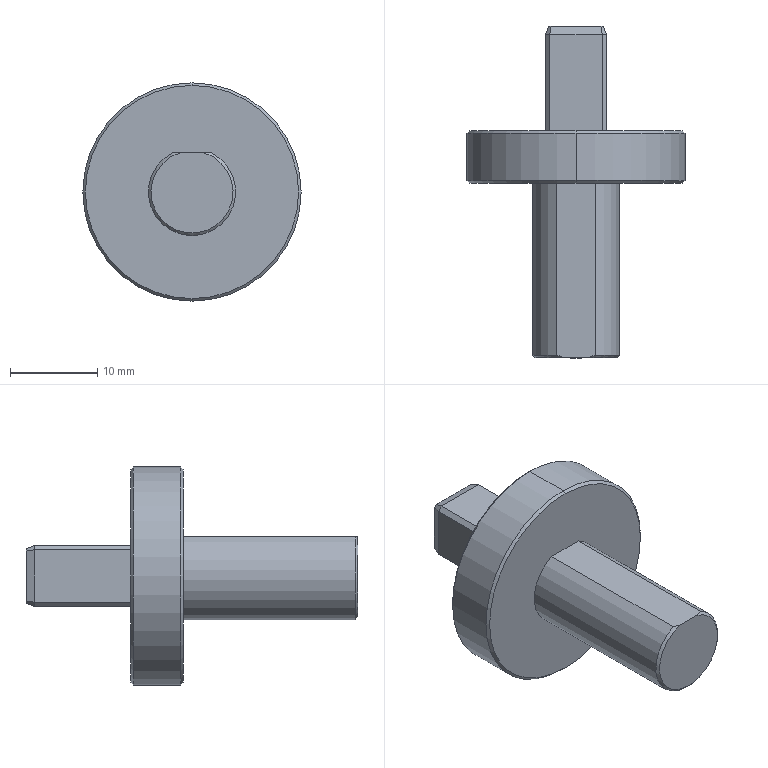Part | NX | features BREP 1 | 1 solid | 29 faces | box 25 x 38 x 25 mm | volume 5056 mm3 | plane 21 | cone 5 | cylinder 3 | commonest cylinder face diameters 25 x2 10 x1
STEP:
#1=CARTESIAN_POINT('',(0.,20.,-12.2));
#2=VERTEX_POINT('',#1);
#3=CARTESIAN_POINT('',(0.,20.,12.2));
#4=VERTEX_POINT('',#3);
#5=CARTESIAN_POINT('',(0.,20.,0.));
#6=DIRECTION('',(0.,-1.,0.));
#7=DIRECTION('',(0.,0.,1.));
#8=AXIS2_PLACEMENT_3D('',#5,#6,#7);
#9=CIRCLE('',#8,12.2);
#10=EDGE_CURVE('',#2,#4,#9,.T.);
#11=ORIENTED_EDGE('',*,*,#10,.F.);
#12=CARTESIAN_POINT('',(0.,20.3,-12.5));
#13=VERTEX_POINT('',#12);
#14=CARTESIAN_POINT('',(0.,20.3,-12.5));
#15=DIRECTION('',(0.,0.7071,-0.7071));
#16=VECTOR('',#15,1000.);
#17=LINE('',#14,#16);
#18=EDGE_CURVE('',#2,#13,#17,.T.);
#19=ORIENTED_EDGE('',*,*,#18,.T.);
#20=CARTESIAN_POINT('',(0.,20.3,12.5));
#21=VERTEX_POINT('',#20);
#22=CARTESIAN_POINT('',(0.,20.3,0.));
#23=DIRECTION('',(0.,1.,0.));
#24=DIRECTION('',(0.,0.,1.));
#25=AXIS2_PLACEMENT_3D('',#22,#23,#24);
#26=CIRCLE('',#25,12.5);
#27=EDGE_CURVE('',#21,#13,#26,.T.);
#28=ORIENTED_EDGE('',*,*,#27,.F.);
#29=CARTESIAN_POINT('',(0.,20.3,12.5));
#30=DIRECTION('',(0.,0.7071,0.7071));
#31=VECTOR('',#30,1000.);
#32=LINE('',#29,#31);
#33=EDGE_CURVE('',#4,#21,#32,.T.);
#34=ORIENTED_EDGE('',*,*,#33,.F.);
#35=EDGE_LOOP('',(#11,#19,#28,#34));
#36=FACE_BOUND('',#35,.T.);
#37=CARTESIAN_POINT('',(0.,20.3,0.));
#38=DIRECTION('',(0.,1.,0.));
#39=DIRECTION('',(0.,0.,-1.));
#40=AXIS2_PLACEMENT_3D('',#37,#38,#39);
#41=CONICAL_SURFACE('',#40,12.5,0.7854);
#42=ADVANCED_FACE('',(#36),#41,.T.);
#43=CARTESIAN_POINT('',(0.,26.,12.2));
#44=VERTEX_POINT('',#43);
#45=CARTESIAN_POINT('',(0.,26.,-12.2));
#46=VERTEX_POINT('',#45);
#47=CARTESIAN_POINT('',(0.,26.,0.));
#48=DIRECTION('',(0.,1.,0.));
#49=DIRECTION('',(0.,0.,1.));
#50=AXIS2_PLACEMENT_3D('',#47,#48,#49);
#51=CIRCLE('',#50,12.2);
#52=EDGE_CURVE('',#44,#46,#51,.T.);
#53=ORIENTED_EDGE('',*,*,#52,.F.);
#54=CARTESIAN_POINT('',(0.,25.7,12.5));
#55=VERTEX_POINT('',#54);
#56=CARTESIAN_POINT('',(0.,26.,12.2));
#57=DIRECTION('',(0.,-0.7071,0.7071));
#58=VECTOR('',#57,1000.);
#59=LINE('',#56,#58);
#60=EDGE_CURVE('',#55,#44,#59,.F.);
#61=ORIENTED_EDGE('',*,*,#60,.F.);
#62=CARTESIAN_POINT('',(0.,25.7,-12.5));
#63=VERTEX_POINT('',#62);
#64=CARTESIAN_POINT('',(0.,25.7,0.));
#65=DIRECTION('',(0.,-1.,0.));
#66=DIRECTION('',(0.,0.,1.));
#67=AXIS2_PLACEMENT_3D('',#64,#65,#66);
#68=CIRCLE('',#67,12.5);
#69=EDGE_CURVE('',#63,#55,#68,.T.);
#70=ORIENTED_EDGE('',*,*,#69,.F.);
#71=CARTESIAN_POINT('',(0.,26.,-12.2));
#72=DIRECTION('',(0.,-0.7071,-0.7071));
#73=VECTOR('',#72,1000.);
#74=LINE('',#71,#73);
#75=EDGE_CURVE('',#63,#46,#74,.F.);
#76=ORIENTED_EDGE('',*,*,#75,.T.);
#77=EDGE_LOOP('',(#53,#61,#70,#76));
#78=FACE_BOUND('',#77,.T.);
#79=CARTESIAN_POINT('',(0.,26.,0.));
#80=DIRECTION('',(0.,-1.,0.));
#81=DIRECTION('',(0.,0.,1.));
#82=AXIS2_PLACEMENT_3D('',#79,#80,#81);
#83=CONICAL_SURFACE('',#82,12.2,0.7854);
#84=ADVANCED_FACE('',(#78),#83,.T.);
#85=ORIENTED_EDGE('',*,*,#27,.T.);
#86=CARTESIAN_POINT('',(0.,66.923,-12.5));
#87=DIRECTION('',(0.,1.,0.));
#88=VECTOR('',#87,1000.);
#89=LINE('',#86,#88);
#90=EDGE_CURVE('',#13,#63,#89,.T.);
#91=ORIENTED_EDGE('',*,*,#90,.T.);
#92=ORIENTED_EDGE('',*,*,#69,.T.);
#93=CARTESIAN_POINT('',(0.,66.923,12.5));
#94=DIRECTION('',(0.,1.,0.));
#95=VECTOR('',#94,1000.);
#96=LINE('',#93,#95);
#97=EDGE_CURVE('',#21,#55,#96,.T.);
#98=ORIENTED_EDGE('',*,*,#97,.F.);
#99=EDGE_LOOP('',(#85,#91,#92,#98));
#100=FACE_BOUND('',#99,.T.);
#101=CARTESIAN_POINT('',(0.,66.923,0.));
#102=DIRECTION('',(0.,1.,0.));
#103=DIRECTION('',(0.,0.,-1.));
#104=AXIS2_PLACEMENT_3D('',#101,#102,#103);
#105=CYLINDRICAL_SURFACE('',#104,12.5);
#106=ADVANCED_FACE('',(#100),#105,.T.);
#107=ORIENTED_EDGE('',*,*,#90,.F.);
#108=CARTESIAN_POINT('',(0.,20.3,0.));
#109=DIRECTION('',(0.,1.,0.));
#110=DIRECTION('',(0.,0.,1.));
#111=AXIS2_PLACEMENT_3D('',#108,#109,#110);
#112=CIRCLE('',#111,12.5);
#113=EDGE_CURVE('',#13,#21,#112,.T.);
#114=ORIENTED_EDGE('',*,*,#113,.T.);
#115=ORIENTED_EDGE('',*,*,#97,.T.);
#116=CARTESIAN_POINT('',(0.,25.7,0.));
#117=DIRECTION('',(0.,-1.,0.));
#118=DIRECTION('',(0.,0.,1.));
#119=AXIS2_PLACEMENT_3D('',#116,#117,#118);
#120=CIRCLE('',#119,12.5);
#121=EDGE_CURVE('',#55,#63,#120,.T.);
#122=ORIENTED_EDGE('',*,*,#121,.T.);
#123=EDGE_LOOP('',(#107,#114,#115,#122));
#124=FACE_BOUND('',#123,.T.);
#125=CARTESIAN_POINT('',(0.,66.923,0.));
#126=DIRECTION('',(0.,1.,0.));
#127=DIRECTION('',(0.,0.,-1.));
#128=AXIS2_PLACEMENT_3D('',#125,#126,#127);
#129=CYLINDRICAL_SURFACE('',#128,12.5);
#130=ADVANCED_FACE('',(#124),#129,.T.);
#131=CARTESIAN_POINT('',(0.,20.,0.));
#132=DIRECTION('',(0.,-1.,0.));
#133=DIRECTION('',(0.,0.,1.));
#134=AXIS2_PLACEMENT_3D('',#131,#132,#133);
#135=CIRCLE('',#134,12.2);
#136=EDGE_CURVE('',#4,#2,#135,.T.);
#137=ORIENTED_EDGE('',*,*,#136,.T.);
#138=ORIENTED_EDGE('',*,*,#10,.T.);
#139=EDGE_LOOP('',(#137,#138));
#140=FACE_BOUND('',#139,.T.);
#141=CARTESIAN_POINT('',(2.179,20.,4.5));
#142=VERTEX_POINT('',#141);
#143=CARTESIAN_POINT('',(-2.179,20.,4.5));
#144=VERTEX_POINT('',#143);
#145=CARTESIAN_POINT('',(0.,20.,0.));
#146=DIRECTION('',(0.,1.,0.));
#147=DIRECTION('',(0.,0.,1.));
#148=AXIS2_PLACEMENT_3D('',#145,#146,#147);
#149=CIRCLE('',#148,5.);
#150=EDGE_CURVE('',#142,#144,#149,.T.);
#151=ORIENTED_EDGE('',*,*,#150,.T.);
#152=CARTESIAN_POINT('',(-2.179,20.,4.5));
#153=DIRECTION('',(1.,0.,0.));
#154=VECTOR('',#153,1000.);
#155=LINE('',#152,#154);
#156=EDGE_CURVE('',#144,#142,#155,.T.);
#157=ORIENTED_EDGE('',*,*,#156,.T.);
#158=EDGE_LOOP('',(#151,#157));
#159=FACE_BOUND('',#158,.T.);
#160=CARTESIAN_POINT('',(12.5,20.,0.));
#161=DIRECTION('',(0.,1.,0.));
#162=DIRECTION('',(0.,0.,-1.));
#163=AXIS2_PLACEMENT_3D('',#160,#161,#162);
#164=PLANE('',#163);
#165=ADVANCED_FACE('',(#140,#159),#164,.F.);
#166=CARTESIAN_POINT('',(2.179,0.3,4.5));
#167=VERTEX_POINT('',#166);
#168=CARTESIAN_POINT('',(2.179,24.387,4.5));
#169=DIRECTION('',(0.,-1.,0.));
#170=VECTOR('',#169,1000.);
#171=LINE('',#168,#170);
#172=EDGE_CURVE('',#167,#142,#171,.F.);
#173=ORIENTED_EDGE('',*,*,#172,.F.);
#174=CARTESIAN_POINT('',(-2.179,0.3,4.5));
#175=VERTEX_POINT('',#174);
#176=CARTESIAN_POINT('',(0.,0.3,0.));
#177=DIRECTION('',(0.,1.,0.));
#178=DIRECTION('',(0.,0.,1.));
#179=AXIS2_PLACEMENT_3D('',#176,#177,#178);
#180=CIRCLE('',#179,5.);
#181=EDGE_CURVE('',#167,#175,#180,.T.);
#182=ORIENTED_EDGE('',*,*,#181,.T.);
#183=CARTESIAN_POINT('',(-2.179,24.387,4.5));
#184=DIRECTION('',(0.,-1.,0.));
#185=VECTOR('',#184,1000.);
#186=LINE('',#183,#185);
#187=EDGE_CURVE('',#175,#144,#186,.F.);
#188=ORIENTED_EDGE('',*,*,#187,.T.);
#189=ORIENTED_EDGE('',*,*,#150,.F.);
#190=EDGE_LOOP('',(#173,#182,#188,#189));
#191=FACE_BOUND('',#190,.T.);
#192=CARTESIAN_POINT('',(0.,66.923,0.));
#193=DIRECTION('',(0.,1.,0.));
#194=DIRECTION('',(0.,0.,-1.));
#195=AXIS2_PLACEMENT_3D('',#192,#193,#194);
#196=CYLINDRICAL_SURFACE('',#195,5.);
#197=ADVANCED_FACE('',(#191),#196,.T.);
#198=CARTESIAN_POINT('',(-1.356,0.,4.5));
#199=VERTEX_POINT('',#198);
#200=CARTESIAN_POINT('',(1.356,0.,4.5));
#201=VERTEX_POINT('',#200);
#202=CARTESIAN_POINT('',(-2.179,0.,4.5));
#203=DIRECTION('',(1.,0.,0.));
#204=VECTOR('',#203,1000.);
#205=LINE('',#202,#204);
#206=EDGE_CURVE('',#199,#201,#205,.T.);
#207=ORIENTED_EDGE('',*,*,#206,.F.);
#208=CARTESIAN_POINT('',(0.,0.,0.));
#209=DIRECTION('',(0.,-1.,0.));
#210=DIRECTION('',(0.,0.,1.));
#211=AXIS2_PLACEMENT_3D('',#208,#209,#210);
#212=CIRCLE('',#211,4.7);
#213=EDGE_CURVE('',#199,#201,#212,.T.);
#214=ORIENTED_EDGE('',*,*,#213,.T.);
#215=EDGE_LOOP('',(#207,#214));
#216=FACE_BOUND('',#215,.T.);
#217=CARTESIAN_POINT('',(5.,0.,0.));
#218=DIRECTION('',(0.,1.,0.));
#219=DIRECTION('',(0.,0.,-1.));
#220=AXIS2_PLACEMENT_3D('',#217,#218,#219);
#221=PLANE('',#220);
#222=ADVANCED_FACE('',(#216),#221,.F.);
#223=ORIENTED_EDGE('',*,*,#187,.F.);
#224=CARTESIAN_POINT('',(-2.179,0.3,4.5));
#225=CARTESIAN_POINT('',(-1.911,0.1831,4.5));
#226=CARTESIAN_POINT('',(-1.638,0.08116,4.5));
#227=CARTESIAN_POINT('',(-1.356,0.,4.5));
#228=B_SPLINE_CURVE_WITH_KNOTS('',3,(#224,#225,#226,#227),.UNSPECIFIED.,.F.,.F.,(4,4),(0.,0.000876),.UNSPECIFIED.);
#229=EDGE_CURVE('',#175,#199,#228,.T.);
#230=ORIENTED_EDGE('',*,*,#229,.T.);
#231=ORIENTED_EDGE('',*,*,#206,.T.);
#232=CARTESIAN_POINT('',(1.356,0.,4.5));
#233=CARTESIAN_POINT('',(1.638,0.08116,4.5));
#234=CARTESIAN_POINT('',(1.911,0.1831,4.5));
#235=CARTESIAN_POINT('',(2.179,0.3,4.5));
#236=B_SPLINE_CURVE_WITH_KNOTS('',3,(#232,#233,#234,#235),.UNSPECIFIED.,.F.,.F.,(4,4),(0.,0.000876),.UNSPECIFIED.);
#237=EDGE_CURVE('',#201,#167,#236,.T.);
#238=ORIENTED_EDGE('',*,*,#237,.T.);
#239=ORIENTED_EDGE('',*,*,#172,.T.);
#240=ORIENTED_EDGE('',*,*,#156,.F.);
#241=EDGE_LOOP('',(#223,#230,#231,#238,#239,#240));
#242=FACE_BOUND('',#241,.T.);
#243=CARTESIAN_POINT('',(-2.179,24.387,4.5));
#244=DIRECTION('',(0.,0.,-1.));
#245=DIRECTION('',(1.,0.,0.));
#246=AXIS2_PLACEMENT_3D('',#243,#244,#245);
#247=PLANE('',#246);
#248=ADVANCED_FACE('',(#242),#247,.F.);
#249=CARTESIAN_POINT('',(0.,26.,0.));
#250=DIRECTION('',(0.,1.,0.));
#251=DIRECTION('',(0.,0.,1.));
#252=AXIS2_PLACEMENT_3D('',#249,#250,#251);
#253=CIRCLE('',#252,12.2);
#254=EDGE_CURVE('',#46,#44,#253,.T.);
#255=ORIENTED_EDGE('',*,*,#254,.T.);
#256=ORIENTED_EDGE('',*,*,#52,.T.);
#257=EDGE_LOOP('',(#255,#256));
#258=FACE_BOUND('',#257,.T.);
#259=CARTESIAN_POINT('',(-3.,26.,3.5));
#260=VERTEX_POINT('',#259);
#261=CARTESIAN_POINT('',(3.,26.,3.5));
#262=VERTEX_POINT('',#261);
#263=CARTESIAN_POINT('',(-3.5,26.,3.5));
#264=DIRECTION('',(1.,0.,0.));
#265=VECTOR('',#264,1000.);
#266=LINE('',#263,#265);
#267=EDGE_CURVE('',#260,#262,#266,.T.);
#268=ORIENTED_EDGE('',*,*,#267,.F.);
#269=CARTESIAN_POINT('',(-3.5,26.,3.));
#270=VERTEX_POINT('',#269);
#271=CARTESIAN_POINT('',(-3.5,26.,3.));
#272=DIRECTION('',(-0.7071,0.,-0.7071));
#273=VECTOR('',#272,1000.);
#274=LINE('',#271,#273);
#275=EDGE_CURVE('',#260,#270,#274,.T.);
#276=ORIENTED_EDGE('',*,*,#275,.T.);
#277=CARTESIAN_POINT('',(-3.5,26.,-3.));
#278=VERTEX_POINT('',#277);
#279=CARTESIAN_POINT('',(-3.5,26.,-3.5));
#280=DIRECTION('',(0.,0.,1.));
#281=VECTOR('',#280,1000.);
#282=LINE('',#279,#281);
#283=EDGE_CURVE('',#278,#270,#282,.T.);
#284=ORIENTED_EDGE('',*,*,#283,.F.);
#285=CARTESIAN_POINT('',(-3.,26.,-3.5));
#286=VERTEX_POINT('',#285);
#287=CARTESIAN_POINT('',(-3.,26.,-3.5));
#288=DIRECTION('',(0.7071,0.,-0.7071));
#289=VECTOR('',#288,1000.);
#290=LINE('',#287,#289);
#291=EDGE_CURVE('',#278,#286,#290,.T.);
#292=ORIENTED_EDGE('',*,*,#291,.T.);
#293=CARTESIAN_POINT('',(3.,26.,-3.5));
#294=VERTEX_POINT('',#293);
#295=CARTESIAN_POINT('',(-3.5,26.,-3.5));
#296=DIRECTION('',(-1.,0.,0.));
#297=VECTOR('',#296,1000.);
#298=LINE('',#295,#297);
#299=EDGE_CURVE('',#294,#286,#298,.T.);
#300=ORIENTED_EDGE('',*,*,#299,.F.);
#301=CARTESIAN_POINT('',(3.5,26.,-3.));
#302=VERTEX_POINT('',#301);
#303=CARTESIAN_POINT('',(3.5,26.,-3.));
#304=DIRECTION('',(0.7071,0.,0.7071));
#305=VECTOR('',#304,1000.);
#306=LINE('',#303,#305);
#307=EDGE_CURVE('',#294,#302,#306,.T.);
#308=ORIENTED_EDGE('',*,*,#307,.T.);
#309=CARTESIAN_POINT('',(3.5,26.,3.));
#310=VERTEX_POINT('',#309);
#311=CARTESIAN_POINT('',(3.5,26.,-3.5));
#312=DIRECTION('',(0.,0.,-1.));
#313=VECTOR('',#312,1000.);
#314=LINE('',#311,#313);
#315=EDGE_CURVE('',#310,#302,#314,.T.);
#316=ORIENTED_EDGE('',*,*,#315,.F.);
#317=CARTESIAN_POINT('',(3.,26.,3.5));
#318=DIRECTION('',(-0.7071,0.,0.7071));
#319=VECTOR('',#318,1000.);
#320=LINE('',#317,#319);
#321=EDGE_CURVE('',#310,#262,#320,.T.);
#322=ORIENTED_EDGE('',*,*,#321,.T.);
#323=EDGE_LOOP('',(#268,#276,#284,#292,#300,#308,#316,#322));
#324=FACE_BOUND('',#323,.T.);
#325=CARTESIAN_POINT('',(0.,26.,0.));
#326=DIRECTION('',(0.,1.,0.));
#327=DIRECTION('',(0.,0.,-1.));
#328=AXIS2_PLACEMENT_3D('',#325,#326,#327);
#329=PLANE('',#328);
#330=ADVANCED_FACE('',(#258,#324),#329,.T.);
#331=CARTESIAN_POINT('',(3.5,37.,-3.));
#332=VERTEX_POINT('',#331);
#333=CARTESIAN_POINT('',(3.5,26.,-3.));
#334=DIRECTION('',(0.,1.,0.));
#335=VECTOR('',#334,1000.);
#336=LINE('',#333,#335);
#337=EDGE_CURVE('',#302,#332,#336,.T.);
#338=ORIENTED_EDGE('',*,*,#337,.T.);
#339=CARTESIAN_POINT('',(3.5,37.,3.));
#340=VERTEX_POINT('',#339);
#341=CARTESIAN_POINT('',(3.5,37.,3.));
#342=DIRECTION('',(0.,0.,1.));
#343=VECTOR('',#342,1000.);
#344=LINE('',#341,#343);
#345=EDGE_CURVE('',#332,#340,#344,.T.);
#346=ORIENTED_EDGE('',*,*,#345,.T.);
#347=CARTESIAN_POINT('',(3.5,26.,3.));
#348=DIRECTION('',(0.,-1.,0.));
#349=VECTOR('',#348,1000.);
#350=LINE('',#347,#349);
#351=EDGE_CURVE('',#340,#310,#350,.T.);
#352=ORIENTED_EDGE('',*,*,#351,.T.);
#353=ORIENTED_EDGE('',*,*,#315,.T.);
#354=EDGE_LOOP('',(#338,#346,#352,#353));
#355=FACE_BOUND('',#354,.T.);
#356=CARTESIAN_POINT('',(3.5,26.,-3.5));
#357=DIRECTION('',(1.,0.,0.));
#358=DIRECTION('',(0.,0.,1.));
#359=AXIS2_PLACEMENT_3D('',#356,#357,#358);
#360=PLANE('',#359);
#361=ADVANCED_FACE('',(#355),#360,.T.);
#362=CARTESIAN_POINT('',(3.,37.,3.5));
#363=VERTEX_POINT('',#362);
#364=CARTESIAN_POINT('',(3.,26.,3.5));
#365=DIRECTION('',(0.,1.,0.));
#366=VECTOR('',#365,1000.);
#367=LINE('',#364,#366);
#368=EDGE_CURVE('',#262,#363,#367,.T.);
#369=ORIENTED_EDGE('',*,*,#368,.T.);
#370=CARTESIAN_POINT('',(-3.,37.,3.5));
#371=VERTEX_POINT('',#370);
#372=CARTESIAN_POINT('',(-3.,37.,3.5));
#373=DIRECTION('',(-1.,0.,0.));
#374=VECTOR('',#373,1000.);
#375=LINE('',#372,#374);
#376=EDGE_CURVE('',#363,#371,#375,.T.);
#377=ORIENTED_EDGE('',*,*,#376,.T.);
#378=CARTESIAN_POINT('',(-3.,26.,3.5));
#379=DIRECTION('',(0.,-1.,0.));
#380=VECTOR('',#379,1000.);
#381=LINE('',#378,#380);
#382=EDGE_CURVE('',#371,#260,#381,.T.);
#383=ORIENTED_EDGE('',*,*,#382,.T.);
#384=ORIENTED_EDGE('',*,*,#267,.T.);
#385=EDGE_LOOP('',(#369,#377,#383,#384));
#386=FACE_BOUND('',#385,.T.);
#387=CARTESIAN_POINT('',(-3.5,26.,3.5));
#388=DIRECTION('',(0.,0.,1.));
#389=DIRECTION('',(-1.,0.,0.));
#390=AXIS2_PLACEMENT_3D('',#387,#388,#389);
#391=PLANE('',#390);
#392=ADVANCED_FACE('',(#386),#391,.T.);
#393=CARTESIAN_POINT('',(-3.5,37.,3.));
#394=VERTEX_POINT('',#393);
#395=CARTESIAN_POINT('',(-3.5,26.,3.));
#396=DIRECTION('',(0.,1.,0.));
#397=VECTOR('',#396,1000.);
#398=LINE('',#395,#397);
#399=EDGE_CURVE('',#270,#394,#398,.T.);
#400=ORIENTED_EDGE('',*,*,#399,.T.);
#401=CARTESIAN_POINT('',(-3.5,37.,-3.));
#402=VERTEX_POINT('',#401);
#403=CARTESIAN_POINT('',(-3.5,37.,-3.));
#404=DIRECTION('',(0.,0.,-1.));
#405=VECTOR('',#404,1000.);
#406=LINE('',#403,#405);
#407=EDGE_CURVE('',#394,#402,#406,.T.);
#408=ORIENTED_EDGE('',*,*,#407,.T.);
#409=CARTESIAN_POINT('',(-3.5,26.,-3.));
#410=DIRECTION('',(0.,-1.,0.));
#411=VECTOR('',#410,1000.);
#412=LINE('',#409,#411);
#413=EDGE_CURVE('',#402,#278,#412,.T.);
#414=ORIENTED_EDGE('',*,*,#413,.T.);
#415=ORIENTED_EDGE('',*,*,#283,.T.);
#416=EDGE_LOOP('',(#400,#408,#414,#415));
#417=FACE_BOUND('',#416,.T.);
#418=CARTESIAN_POINT('',(-3.5,26.,-3.5));
#419=DIRECTION('',(-1.,0.,0.));
#420=DIRECTION('',(0.,0.,-1.));
#421=AXIS2_PLACEMENT_3D('',#418,#419,#420);
#422=PLANE('',#421);
#423=ADVANCED_FACE('',(#417),#422,.T.);
#424=CARTESIAN_POINT('',(-3.,37.,-3.5));
#425=VERTEX_POINT('',#424);
#426=CARTESIAN_POINT('',(-3.,26.,-3.5));
#427=DIRECTION('',(0.,1.,0.));
#428=VECTOR('',#427,1000.);
#429=LINE('',#426,#428);
#430=EDGE_CURVE('',#286,#425,#429,.T.);
#431=ORIENTED_EDGE('',*,*,#430,.T.);
#432=CARTESIAN_POINT('',(3.,37.,-3.5));
#433=VERTEX_POINT('',#432);
#434=CARTESIAN_POINT('',(3.,37.,-3.5));
#435=DIRECTION('',(1.,0.,0.));
#436=VECTOR('',#435,1000.);
#437=LINE('',#434,#436);
#438=EDGE_CURVE('',#425,#433,#437,.T.);
#439=ORIENTED_EDGE('',*,*,#438,.T.);
#440=CARTESIAN_POINT('',(3.,26.,-3.5));
#441=DIRECTION('',(0.,-1.,0.));
#442=VECTOR('',#441,1000.);
#443=LINE('',#440,#442);
#444=EDGE_CURVE('',#433,#294,#443,.T.);
#445=ORIENTED_EDGE('',*,*,#444,.T.);
#446=ORIENTED_EDGE('',*,*,#299,.T.);
#447=EDGE_LOOP('',(#431,#439,#445,#446));
#448=FACE_BOUND('',#447,.T.);
#449=CARTESIAN_POINT('',(-3.5,26.,-3.5));
#450=DIRECTION('',(0.,0.,-1.));
#451=DIRECTION('',(1.,0.,0.));
#452=AXIS2_PLACEMENT_3D('',#449,#450,#451);
#453=PLANE('',#452);
#454=ADVANCED_FACE('',(#448),#453,.T.);
#455=CARTESIAN_POINT('',(3.136,38.,2.849));
#456=VERTEX_POINT('',#455);
#457=CARTESIAN_POINT('',(3.136,38.,-2.849));
#458=VERTEX_POINT('',#457);
#459=CARTESIAN_POINT('',(3.136,38.,-3.));
#460=DIRECTION('',(0.,0.,-1.));
#461=VECTOR('',#460,1000.);
#462=LINE('',#459,#461);
#463=EDGE_CURVE('',#456,#458,#462,.T.);
#464=ORIENTED_EDGE('',*,*,#463,.T.);
#465=CARTESIAN_POINT('',(2.849,38.,-3.136));
#466=VERTEX_POINT('',#465);
#467=CARTESIAN_POINT('',(2.743,38.,-3.243));
#468=DIRECTION('',(-0.7071,0.,-0.7071));
#469=VECTOR('',#468,1000.);
#470=LINE('',#467,#469);
#471=EDGE_CURVE('',#458,#466,#470,.T.);
#472=ORIENTED_EDGE('',*,*,#471,.T.);
#473=CARTESIAN_POINT('',(-2.849,38.,-3.136));
#474=VERTEX_POINT('',#473);
#475=CARTESIAN_POINT('',(-3.,38.,-3.136));
#476=DIRECTION('',(-1.,0.,0.));
#477=VECTOR('',#476,1000.);
#478=LINE('',#475,#477);
#479=EDGE_CURVE('',#466,#474,#478,.T.);
#480=ORIENTED_EDGE('',*,*,#479,.T.);
#481=CARTESIAN_POINT('',(-3.136,38.,-2.849));
#482=VERTEX_POINT('',#481);
#483=CARTESIAN_POINT('',(-3.243,38.,-2.743));
#484=DIRECTION('',(-0.7071,0.,0.7071));
#485=VECTOR('',#484,1000.);
#486=LINE('',#483,#485);
#487=EDGE_CURVE('',#474,#482,#486,.T.);
#488=ORIENTED_EDGE('',*,*,#487,.T.);
#489=CARTESIAN_POINT('',(-3.136,38.,2.849));
#490=VERTEX_POINT('',#489);
#491=CARTESIAN_POINT('',(-3.136,38.,3.));
#492=DIRECTION('',(0.,0.,1.));
#493=VECTOR('',#492,1000.);
#494=LINE('',#491,#493);
#495=EDGE_CURVE('',#482,#490,#494,.T.);
#496=ORIENTED_EDGE('',*,*,#495,.T.);
#497=CARTESIAN_POINT('',(-2.849,38.,3.136));
#498=VERTEX_POINT('',#497);
#499=CARTESIAN_POINT('',(-2.743,38.,3.243));
#500=DIRECTION('',(0.7071,0.,0.7071));
#501=VECTOR('',#500,1000.);
#502=LINE('',#499,#501);
#503=EDGE_CURVE('',#490,#498,#502,.T.);
#504=ORIENTED_EDGE('',*,*,#503,.T.);
#505=CARTESIAN_POINT('',(2.849,38.,3.136));
#506=VERTEX_POINT('',#505);
#507=CARTESIAN_POINT('',(3.,38.,3.136));
#508=DIRECTION('',(1.,0.,0.));
#509=VECTOR('',#508,1000.);
#510=LINE('',#507,#509);
#511=EDGE_CURVE('',#498,#506,#510,.T.);
#512=ORIENTED_EDGE('',*,*,#511,.T.);
#513=CARTESIAN_POINT('',(3.243,38.,2.743));
#514=DIRECTION('',(0.7071,0.,-0.7071));
#515=VECTOR('',#514,1000.);
#516=LINE('',#513,#515);
#517=EDGE_CURVE('',#506,#456,#516,.T.);
#518=ORIENTED_EDGE('',*,*,#517,.T.);
#519=EDGE_LOOP('',(#464,#472,#480,#488,#496,#504,#512,#518));
#520=FACE_BOUND('',#519,.T.);
#521=CARTESIAN_POINT('',(0.,38.,0.));
#522=DIRECTION('',(0.,-1.,0.));
#523=DIRECTION('',(0.,0.,1.));
#524=AXIS2_PLACEMENT_3D('',#521,#522,#523);
#525=PLANE('',#524);
#526=ADVANCED_FACE('',(#520),#525,.F.);
#527=ORIENTED_EDGE('',*,*,#413,.F.);
#528=CARTESIAN_POINT('',(-3.,37.,-3.5));
#529=DIRECTION('',(0.7071,0.,-0.7071));
#530=VECTOR('',#529,1000.);
#531=LINE('',#528,#530);
#532=EDGE_CURVE('',#402,#425,#531,.T.);
#533=ORIENTED_EDGE('',*,*,#532,.T.);
#534=ORIENTED_EDGE('',*,*,#430,.F.);
#535=ORIENTED_EDGE('',*,*,#291,.F.);
#536=EDGE_LOOP('',(#527,#533,#534,#535));
#537=FACE_BOUND('',#536,.T.);
#538=CARTESIAN_POINT('',(-3.,26.,-3.5));
#539=DIRECTION('',(0.7071,0.,0.7071));
#540=DIRECTION('',(0.,-1.,0.));
#541=AXIS2_PLACEMENT_3D('',#538,#539,#540);
#542=PLANE('',#541);
#543=ADVANCED_FACE('',(#537),#542,.F.);
#544=ORIENTED_EDGE('',*,*,#444,.F.);
#545=CARTESIAN_POINT('',(3.5,37.,-3.));
#546=DIRECTION('',(0.7071,0.,0.7071));
#547=VECTOR('',#546,1000.);
#548=LINE('',#545,#547);
#549=EDGE_CURVE('',#433,#332,#548,.T.);
#550=ORIENTED_EDGE('',*,*,#549,.T.);
#551=ORIENTED_EDGE('',*,*,#337,.F.);
#552=ORIENTED_EDGE('',*,*,#307,.F.);
#553=EDGE_LOOP('',(#544,#550,#551,#552));
#554=FACE_BOUND('',#553,.T.);
#555=CARTESIAN_POINT('',(3.5,26.,-3.));
#556=DIRECTION('',(-0.7071,0.,0.7071));
#557=DIRECTION('',(0.,-1.,0.));
#558=AXIS2_PLACEMENT_3D('',#555,#556,#557);
#559=PLANE('',#558);
#560=ADVANCED_FACE('',(#554),#559,.F.);
#561=ORIENTED_EDGE('',*,*,#351,.F.);
#562=CARTESIAN_POINT('',(3.,37.,3.5));
#563=DIRECTION('',(-0.7071,0.,0.7071));
#564=VECTOR('',#563,1000.);
#565=LINE('',#562,#564);
#566=EDGE_CURVE('',#340,#363,#565,.T.);
#567=ORIENTED_EDGE('',*,*,#566,.T.);
#568=ORIENTED_EDGE('',*,*,#368,.F.);
#569=ORIENTED_EDGE('',*,*,#321,.F.);
#570=EDGE_LOOP('',(#561,#567,#568,#569));
#571=FACE_BOUND('',#570,.T.);
#572=CARTESIAN_POINT('',(3.,26.,3.5));
#573=DIRECTION('',(-0.7071,0.,-0.7071));
#574=DIRECTION('',(0.,-1.,0.));
#575=AXIS2_PLACEMENT_3D('',#572,#573,#574);
#576=PLANE('',#575);
#577=ADVANCED_FACE('',(#571),#576,.F.);
#578=ORIENTED_EDGE('',*,*,#382,.F.);
#579=CARTESIAN_POINT('',(-3.5,37.,3.));
#580=DIRECTION('',(-0.7071,0.,-0.7071));
#581=VECTOR('',#580,1000.);
#582=LINE('',#579,#581);
#583=EDGE_CURVE('',#371,#394,#582,.T.);
#584=ORIENTED_EDGE('',*,*,#583,.T.);
#585=ORIENTED_EDGE('',*,*,#399,.F.);
#586=ORIENTED_EDGE('',*,*,#275,.F.);
#587=EDGE_LOOP('',(#578,#584,#585,#586));
#588=FACE_BOUND('',#587,.T.);
#589=CARTESIAN_POINT('',(-3.5,26.,3.));
#590=DIRECTION('',(0.7071,0.,-0.7071));
#591=DIRECTION('',(0.,-1.,0.));
#592=AXIS2_PLACEMENT_3D('',#589,#590,#591);
#593=PLANE('',#592);
#594=ADVANCED_FACE('',(#588),#593,.F.);
#595=CARTESIAN_POINT('',(-3.001,38.372,2.793));
#596=DIRECTION('',(0.3386,0.9304,-0.1403));
#597=VECTOR('',#596,1000.);
#598=LINE('',#595,#597);
#599=EDGE_CURVE('',#394,#490,#598,.T.);
#600=ORIENTED_EDGE('',*,*,#599,.F.);
#601=ORIENTED_EDGE('',*,*,#583,.F.);
#602=CARTESIAN_POINT('',(-2.845,38.026,3.126));
#603=DIRECTION('',(-0.1403,-0.9304,0.3386));
#604=VECTOR('',#603,1000.);
#605=LINE('',#602,#604);
#606=EDGE_CURVE('',#498,#371,#605,.T.);
#607=ORIENTED_EDGE('',*,*,#606,.F.);
#608=ORIENTED_EDGE('',*,*,#503,.F.);
#609=EDGE_LOOP('',(#600,#601,#607,#608));
#610=FACE_BOUND('',#609,.T.);
#611=CARTESIAN_POINT('',(-2.993,38.,2.993));
#612=DIRECTION('',(0.6645,-0.342,-0.6645));
#613=DIRECTION('',(-0.7071,0.,-0.7071));
#614=AXIS2_PLACEMENT_3D('',#611,#612,#613);
#615=PLANE('',#614);
#616=ADVANCED_FACE('',(#610),#615,.F.);
#617=ORIENTED_EDGE('',*,*,#606,.T.);
#618=ORIENTED_EDGE('',*,*,#376,.F.);
#619=CARTESIAN_POINT('',(2.793,38.372,3.001));
#620=DIRECTION('',(0.1403,-0.9304,0.3386));
#621=VECTOR('',#620,1000.);
#622=LINE('',#619,#621);
#623=EDGE_CURVE('',#506,#363,#622,.T.);
#624=ORIENTED_EDGE('',*,*,#623,.F.);
#625=ORIENTED_EDGE('',*,*,#511,.F.);
#626=EDGE_LOOP('',(#617,#618,#624,#625));
#627=FACE_BOUND('',#626,.T.);
#628=CARTESIAN_POINT('',(0.,38.,3.136));
#629=DIRECTION('',(0.,0.342,0.9397));
#630=DIRECTION('',(1.,0.,0.));
#631=AXIS2_PLACEMENT_3D('',#628,#629,#630);
#632=PLANE('',#631);
#633=ADVANCED_FACE('',(#627),#632,.T.);
#634=ORIENTED_EDGE('',*,*,#599,.T.);
#635=ORIENTED_EDGE('',*,*,#495,.F.);
#636=CARTESIAN_POINT('',(-3.126,38.026,-2.845));
#637=DIRECTION('',(0.3386,0.9304,0.1403));
#638=VECTOR('',#637,1000.);
#639=LINE('',#636,#638);
#640=EDGE_CURVE('',#402,#482,#639,.T.);
#641=ORIENTED_EDGE('',*,*,#640,.F.);
#642=ORIENTED_EDGE('',*,*,#407,.F.);
#643=EDGE_LOOP('',(#634,#635,#641,#642));
#644=FACE_BOUND('',#643,.T.);
#645=CARTESIAN_POINT('',(-3.136,38.,0.));
#646=DIRECTION('',(-0.9397,0.342,0.));
#647=DIRECTION('',(0.,0.,1.));
#648=AXIS2_PLACEMENT_3D('',#645,#646,#647);
#649=PLANE('',#648);
#650=ADVANCED_FACE('',(#644),#649,.T.);
#651=ORIENTED_EDGE('',*,*,#623,.T.);
#652=ORIENTED_EDGE('',*,*,#566,.F.);
#653=CARTESIAN_POINT('',(3.126,38.026,2.845));
#654=DIRECTION('',(0.3386,-0.9304,0.1403));
#655=VECTOR('',#654,1000.);
#656=LINE('',#653,#655);
#657=EDGE_CURVE('',#456,#340,#656,.T.);
#658=ORIENTED_EDGE('',*,*,#657,.F.);
#659=ORIENTED_EDGE('',*,*,#517,.F.);
#660=EDGE_LOOP('',(#651,#652,#658,#659));
#661=FACE_BOUND('',#660,.T.);
#662=CARTESIAN_POINT('',(2.993,38.,2.993));
#663=DIRECTION('',(-0.6645,-0.342,-0.6645));
#664=DIRECTION('',(-0.7071,0.,0.7071));
#665=AXIS2_PLACEMENT_3D('',#662,#663,#664);
#666=PLANE('',#665);
#667=ADVANCED_FACE('',(#661),#666,.F.);
#668=ORIENTED_EDGE('',*,*,#640,.T.);
#669=ORIENTED_EDGE('',*,*,#487,.F.);
#670=CARTESIAN_POINT('',(-2.793,38.372,-3.001));
#671=DIRECTION('',(0.1403,0.9304,0.3386));
#672=VECTOR('',#671,1000.);
#673=LINE('',#670,#672);
#674=EDGE_CURVE('',#425,#474,#673,.T.);
#675=ORIENTED_EDGE('',*,*,#674,.F.);
#676=ORIENTED_EDGE('',*,*,#532,.F.);
#677=EDGE_LOOP('',(#668,#669,#675,#676));
#678=FACE_BOUND('',#677,.T.);
#679=CARTESIAN_POINT('',(-2.993,38.,-2.993));
#680=DIRECTION('',(0.6645,-0.342,0.6645));
#681=DIRECTION('',(0.7071,0.,-0.7071));
#682=AXIS2_PLACEMENT_3D('',#679,#680,#681);
#683=PLANE('',#682);
#684=ADVANCED_FACE('',(#678),#683,.F.);
#685=ORIENTED_EDGE('',*,*,#657,.T.);
#686=ORIENTED_EDGE('',*,*,#345,.F.);
#687=CARTESIAN_POINT('',(3.001,38.372,-2.793));
#688=DIRECTION('',(0.3386,-0.9304,-0.1403));
#689=VECTOR('',#688,1000.);
#690=LINE('',#687,#689);
#691=EDGE_CURVE('',#458,#332,#690,.T.);
#692=ORIENTED_EDGE('',*,*,#691,.F.);
#693=ORIENTED_EDGE('',*,*,#463,.F.);
#694=EDGE_LOOP('',(#685,#686,#692,#693));
#695=FACE_BOUND('',#694,.T.);
#696=CARTESIAN_POINT('',(3.136,38.,0.));
#697=DIRECTION('',(0.9397,0.342,0.));
#698=DIRECTION('',(0.,0.,-1.));
#699=AXIS2_PLACEMENT_3D('',#696,#697,#698);
#700=PLANE('',#699);
#701=ADVANCED_FACE('',(#695),#700,.T.);
#702=ORIENTED_EDGE('',*,*,#674,.T.);
#703=ORIENTED_EDGE('',*,*,#479,.F.);
#704=CARTESIAN_POINT('',(2.793,38.372,-3.001));
#705=DIRECTION('',(-0.1403,0.9304,0.3386));
#706=VECTOR('',#705,1000.);
#707=LINE('',#704,#706);
#708=EDGE_CURVE('',#433,#466,#707,.T.);
#709=ORIENTED_EDGE('',*,*,#708,.F.);
#710=ORIENTED_EDGE('',*,*,#438,.F.);
#711=EDGE_LOOP('',(#702,#703,#709,#710));
#712=FACE_BOUND('',#711,.T.);
#713=CARTESIAN_POINT('',(0.,38.,-3.136));
#714=DIRECTION('',(0.,0.342,-0.9397));
#715=DIRECTION('',(-1.,0.,0.));
#716=AXIS2_PLACEMENT_3D('',#713,#714,#715);
#717=PLANE('',#716);
#718=ADVANCED_FACE('',(#712),#717,.T.);
#719=ORIENTED_EDGE('',*,*,#691,.T.);
#720=ORIENTED_EDGE('',*,*,#549,.F.);
#721=ORIENTED_EDGE('',*,*,#708,.T.);
#722=ORIENTED_EDGE('',*,*,#471,.F.);
#723=EDGE_LOOP('',(#719,#720,#721,#722));
#724=FACE_BOUND('',#723,.T.);
#725=CARTESIAN_POINT('',(2.993,38.,-2.993));
#726=DIRECTION('',(-0.6645,-0.342,0.6645));
#727=DIRECTION('',(0.7071,0.,0.7071));
#728=AXIS2_PLACEMENT_3D('',#725,#726,#727);
#729=PLANE('',#728);
#730=ADVANCED_FACE('',(#724),#729,.F.);
#731=ORIENTED_EDGE('',*,*,#60,.T.);
#732=ORIENTED_EDGE('',*,*,#254,.F.);
#733=ORIENTED_EDGE('',*,*,#75,.F.);
#734=ORIENTED_EDGE('',*,*,#121,.F.);
#735=EDGE_LOOP('',(#731,#732,#733,#734));
#736=FACE_BOUND('',#735,.T.);
#737=CARTESIAN_POINT('',(0.,26.,0.));
#738=DIRECTION('',(0.,-1.,0.));
#739=DIRECTION('',(0.,0.,1.));
#740=AXIS2_PLACEMENT_3D('',#737,#738,#739);
#741=CONICAL_SURFACE('',#740,12.2,0.7854);
#742=ADVANCED_FACE('',(#736),#741,.T.);
#743=ORIENTED_EDGE('',*,*,#18,.F.);
#744=ORIENTED_EDGE('',*,*,#136,.F.);
#745=ORIENTED_EDGE('',*,*,#33,.T.);
#746=ORIENTED_EDGE('',*,*,#113,.F.);
#747=EDGE_LOOP('',(#743,#744,#745,#746));
#748=FACE_BOUND('',#747,.T.);
#749=CARTESIAN_POINT('',(0.,20.3,0.));
#750=DIRECTION('',(0.,1.,0.));
#751=DIRECTION('',(0.,0.,-1.));
#752=AXIS2_PLACEMENT_3D('',#749,#750,#751);
#753=CONICAL_SURFACE('',#752,12.5,0.7854);
#754=ADVANCED_FACE('',(#748),#753,.T.);
#755=ORIENTED_EDGE('',*,*,#237,.F.);
#756=ORIENTED_EDGE('',*,*,#213,.F.);
#757=ORIENTED_EDGE('',*,*,#229,.F.);
#758=ORIENTED_EDGE('',*,*,#181,.F.);
#759=EDGE_LOOP('',(#755,#756,#757,#758));
#760=FACE_BOUND('',#759,.T.);
#761=CARTESIAN_POINT('',(0.,0.3,0.));
#762=DIRECTION('',(0.,1.,0.));
#763=DIRECTION('',(0.,0.,-1.));
#764=AXIS2_PLACEMENT_3D('',#761,#762,#763);
#765=CONICAL_SURFACE('',#764,5.,0.7854);
#766=ADVANCED_FACE('',(#760),#765,.T.);
#767=CLOSED_SHELL('',(#42,#84,#106,#130,#165,#197,#222,#248,#330,#361,#392,#423,#454,#526,#543,#560,#577,#594,#616,#633,#650,#667,#684,#701,#718,#730,#742,#754,#766));
#768=MANIFOLD_SOLID_BREP('',#767);
#769=(LENGTH_UNIT()NAMED_UNIT(*)SI_UNIT(.MILLI.,.METRE.));
#770=UNCERTAINTY_MEASURE_WITH_UNIT(LENGTH_MEASURE(0.0508),#769,'','');
#771=(NAMED_UNIT(*)PLANE_ANGLE_UNIT()SI_UNIT($,.RADIAN.));
#772=(NAMED_UNIT(*)SI_UNIT($,.STERADIAN.)SOLID_ANGLE_UNIT());
#773=(GEOMETRIC_REPRESENTATION_CONTEXT(3)GLOBAL_UNCERTAINTY_ASSIGNED_CONTEXT((#770))GLOBAL_UNIT_ASSIGNED_CONTEXT((#769,#771,#772))REPRESENTATION_CONTEXT('',''));
#774=ADVANCED_BREP_SHAPE_REPRESENTATION('',(#768),#773);